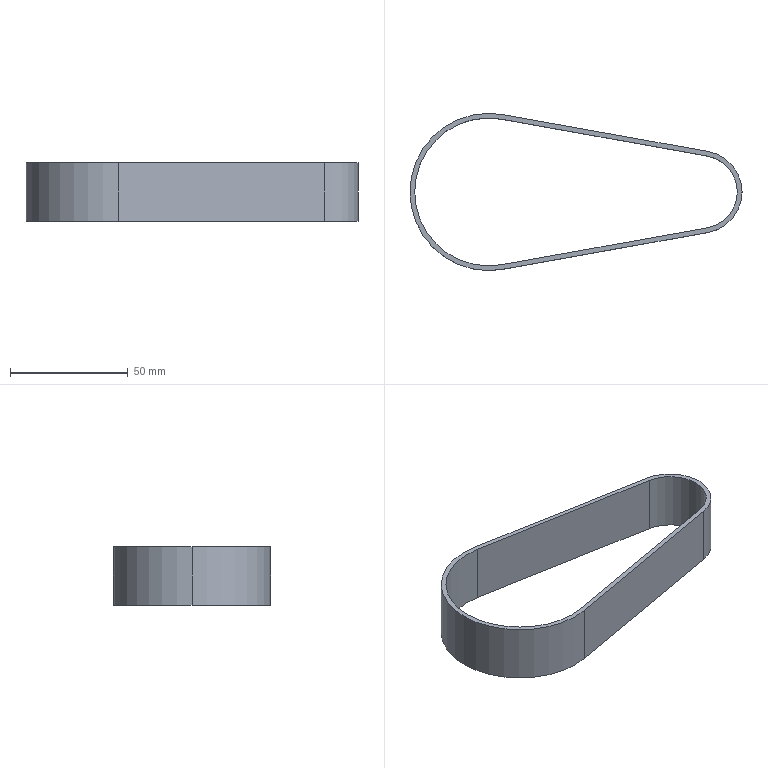Part | SolidWorks | features BaseBody 1 | 1 solid | 12 faces | box 140.79 x 66.7 x 25 mm | volume 16805 mm3 | cylinder 6 | plane 6 | commonest cylinder face diameters 62.7 x2 66.7 x2 30.88 x1 34.88 x1
STEP:
#1=CARTESIAN_POINT('',(-212.674,0.,25.));
#2=VERTEX_POINT('',#1);
#3=CARTESIAN_POINT('',(-175.782,30.856,25.));
#4=VERTEX_POINT('',#3);
#5=CARTESIAN_POINT('',(-181.324,0.,25.));
#6=DIRECTION('',(0.,0.,-1.));
#7=DIRECTION('',(-1.,0.,0.));
#8=AXIS2_PLACEMENT_3D('',#5,#6,#7);
#9=CIRCLE('',#8,31.35);
#10=EDGE_CURVE('',#2,#4,#9,.T.);
#11=ORIENTED_EDGE('',*,*,#10,.F.);
#12=CARTESIAN_POINT('',(-212.674,0.,0.));
#13=VERTEX_POINT('',#12);
#14=CARTESIAN_POINT('',(-212.674,0.,25.));
#15=DIRECTION('',(0.,0.,-1.));
#16=VECTOR('',#15,1000.);
#17=LINE('',#14,#16);
#18=EDGE_CURVE('',#2,#13,#17,.T.);
#19=ORIENTED_EDGE('',*,*,#18,.T.);
#20=CARTESIAN_POINT('',(-175.782,30.856,0.));
#21=VERTEX_POINT('',#20);
#22=CARTESIAN_POINT('',(-181.324,0.,0.));
#23=DIRECTION('',(0.,0.,1.));
#24=DIRECTION('',(-1.,0.,0.));
#25=AXIS2_PLACEMENT_3D('',#22,#23,#24);
#26=CIRCLE('',#25,31.35);
#27=EDGE_CURVE('',#21,#13,#26,.T.);
#28=ORIENTED_EDGE('',*,*,#27,.F.);
#29=CARTESIAN_POINT('',(-175.782,30.856,25.));
#30=DIRECTION('',(0.,0.,-1.));
#31=VECTOR('',#30,1000.);
#32=LINE('',#29,#31);
#33=EDGE_CURVE('',#4,#21,#32,.T.);
#34=ORIENTED_EDGE('',*,*,#33,.F.);
#35=EDGE_LOOP('',(#11,#19,#28,#34));
#36=FACE_OUTER_BOUND('',#35,.T.);
#37=CARTESIAN_POINT('',(-181.324,0.,25.));
#38=DIRECTION('',(0.,0.,-1.));
#39=DIRECTION('',(-1.,0.,0.));
#40=AXIS2_PLACEMENT_3D('',#37,#38,#39);
#41=CYLINDRICAL_SURFACE('',#40,31.35);
#42=ADVANCED_FACE('',(#36),#41,.F.);
#43=CARTESIAN_POINT('',(-214.674,0.,25.));
#44=VERTEX_POINT('',#43);
#45=CARTESIAN_POINT('',(-175.428,-32.825,25.));
#46=VERTEX_POINT('',#45);
#47=CARTESIAN_POINT('',(-181.324,0.,25.));
#48=DIRECTION('',(0.,0.,1.));
#49=DIRECTION('',(-1.,0.,0.));
#50=AXIS2_PLACEMENT_3D('',#47,#48,#49);
#51=CIRCLE('',#50,33.35);
#52=EDGE_CURVE('',#44,#46,#51,.T.);
#53=ORIENTED_EDGE('',*,*,#52,.F.);
#54=CARTESIAN_POINT('',(-214.674,0.,0.));
#55=VERTEX_POINT('',#54);
#56=CARTESIAN_POINT('',(-214.674,0.,25.));
#57=DIRECTION('',(0.,0.,-1.));
#58=VECTOR('',#57,1000.);
#59=LINE('',#56,#58);
#60=EDGE_CURVE('',#44,#55,#59,.T.);
#61=ORIENTED_EDGE('',*,*,#60,.T.);
#62=CARTESIAN_POINT('',(-175.428,-32.825,0.));
#63=VERTEX_POINT('',#62);
#64=CARTESIAN_POINT('',(-181.324,0.,0.));
#65=DIRECTION('',(0.,0.,1.));
#66=DIRECTION('',(-1.,0.,0.));
#67=AXIS2_PLACEMENT_3D('',#64,#65,#66);
#68=CIRCLE('',#67,33.35);
#69=EDGE_CURVE('',#55,#63,#68,.T.);
#70=ORIENTED_EDGE('',*,*,#69,.T.);
#71=CARTESIAN_POINT('',(-175.428,-32.825,25.));
#72=DIRECTION('',(0.,0.,1.));
#73=VECTOR('',#72,1000.);
#74=LINE('',#71,#73);
#75=EDGE_CURVE('',#63,#46,#74,.T.);
#76=ORIENTED_EDGE('',*,*,#75,.T.);
#77=EDGE_LOOP('',(#53,#61,#70,#76));
#78=FACE_OUTER_BOUND('',#77,.T.);
#79=CARTESIAN_POINT('',(-181.324,0.,25.));
#80=DIRECTION('',(0.,0.,-1.));
#81=DIRECTION('',(-1.,0.,0.));
#82=AXIS2_PLACEMENT_3D('',#79,#80,#81);
#83=CYLINDRICAL_SURFACE('',#82,33.35);
#84=ADVANCED_FACE('',(#78),#83,.T.);
#85=CARTESIAN_POINT('',(-175.782,-30.856,25.));
#86=VERTEX_POINT('',#85);
#87=CARTESIAN_POINT('',(-88.594,-15.197,25.));
#88=VERTEX_POINT('',#87);
#89=CARTESIAN_POINT('',(-175.782,-30.856,25.));
#90=DIRECTION('',(0.9843,0.1768,0.));
#91=VECTOR('',#90,1000.);
#92=LINE('',#89,#91);
#93=EDGE_CURVE('',#86,#88,#92,.T.);
#94=ORIENTED_EDGE('',*,*,#93,.T.);
#95=CARTESIAN_POINT('',(-88.594,-15.197,0.));
#96=VERTEX_POINT('',#95);
#97=CARTESIAN_POINT('',(-88.594,-15.197,25.));
#98=DIRECTION('',(0.,0.,-1.));
#99=VECTOR('',#98,1000.);
#100=LINE('',#97,#99);
#101=EDGE_CURVE('',#88,#96,#100,.T.);
#102=ORIENTED_EDGE('',*,*,#101,.T.);
#103=CARTESIAN_POINT('',(-175.782,-30.856,0.));
#104=VERTEX_POINT('',#103);
#105=CARTESIAN_POINT('',(-175.782,-30.856,0.));
#106=DIRECTION('',(-0.9843,-0.1768,0.));
#107=VECTOR('',#106,1000.);
#108=LINE('',#105,#107);
#109=EDGE_CURVE('',#96,#104,#108,.T.);
#110=ORIENTED_EDGE('',*,*,#109,.T.);
#111=CARTESIAN_POINT('',(-175.782,-30.856,25.));
#112=DIRECTION('',(0.,0.,1.));
#113=VECTOR('',#112,1000.);
#114=LINE('',#111,#113);
#115=EDGE_CURVE('',#104,#86,#114,.T.);
#116=ORIENTED_EDGE('',*,*,#115,.T.);
#117=EDGE_LOOP('',(#94,#102,#110,#116));
#118=FACE_OUTER_BOUND('',#117,.T.);
#119=CARTESIAN_POINT('',(-175.782,-30.856,25.));
#120=DIRECTION('',(-0.1768,0.9843,0.));
#121=DIRECTION('',(-0.9843,-0.1768,0.));
#122=AXIS2_PLACEMENT_3D('',#119,#120,#121);
#123=PLANE('',#122);
#124=ADVANCED_FACE('',(#118),#123,.T.);
#125=ORIENTED_EDGE('',*,*,#101,.F.);
#126=CARTESIAN_POINT('',(-88.594,15.197,25.));
#127=VERTEX_POINT('',#126);
#128=CARTESIAN_POINT('',(-91.324,0.,25.));
#129=DIRECTION('',(0.,0.,-1.));
#130=DIRECTION('',(-1.,0.,0.));
#131=AXIS2_PLACEMENT_3D('',#128,#129,#130);
#132=CIRCLE('',#131,15.44);
#133=EDGE_CURVE('',#127,#88,#132,.T.);
#134=ORIENTED_EDGE('',*,*,#133,.F.);
#135=CARTESIAN_POINT('',(-88.594,15.197,0.));
#136=VERTEX_POINT('',#135);
#137=CARTESIAN_POINT('',(-88.594,15.197,25.));
#138=DIRECTION('',(0.,0.,1.));
#139=VECTOR('',#138,1000.);
#140=LINE('',#137,#139);
#141=EDGE_CURVE('',#136,#127,#140,.T.);
#142=ORIENTED_EDGE('',*,*,#141,.F.);
#143=CARTESIAN_POINT('',(-91.324,0.,0.));
#144=DIRECTION('',(0.,0.,1.));
#145=DIRECTION('',(-1.,0.,0.));
#146=AXIS2_PLACEMENT_3D('',#143,#144,#145);
#147=CIRCLE('',#146,15.44);
#148=EDGE_CURVE('',#96,#136,#147,.T.);
#149=ORIENTED_EDGE('',*,*,#148,.F.);
#150=EDGE_LOOP('',(#125,#134,#142,#149));
#151=FACE_OUTER_BOUND('',#150,.T.);
#152=CARTESIAN_POINT('',(-91.324,0.,25.));
#153=DIRECTION('',(0.,0.,-1.));
#154=DIRECTION('',(-1.,0.,0.));
#155=AXIS2_PLACEMENT_3D('',#152,#153,#154);
#156=CYLINDRICAL_SURFACE('',#155,15.44);
#157=ADVANCED_FACE('',(#151),#156,.F.);
#158=CARTESIAN_POINT('',(-175.782,30.856,25.));
#159=DIRECTION('',(0.9843,-0.1768,0.));
#160=VECTOR('',#159,1000.);
#161=LINE('',#158,#160);
#162=EDGE_CURVE('',#4,#127,#161,.T.);
#163=ORIENTED_EDGE('',*,*,#162,.T.);
#164=ORIENTED_EDGE('',*,*,#133,.T.);
#165=ORIENTED_EDGE('',*,*,#93,.F.);
#166=CARTESIAN_POINT('',(-181.324,0.,25.));
#167=DIRECTION('',(0.,0.,-1.));
#168=DIRECTION('',(-1.,0.,0.));
#169=AXIS2_PLACEMENT_3D('',#166,#167,#168);
#170=CIRCLE('',#169,31.35);
#171=EDGE_CURVE('',#86,#2,#170,.T.);
#172=ORIENTED_EDGE('',*,*,#171,.T.);
#173=ORIENTED_EDGE('',*,*,#10,.T.);
#174=EDGE_LOOP('',(#163,#164,#165,#172,#173));
#175=FACE_BOUND('',#174,.T.);
#176=CARTESIAN_POINT('',(-88.241,-17.165,25.));
#177=VERTEX_POINT('',#176);
#178=CARTESIAN_POINT('',(-88.241,17.165,25.));
#179=VERTEX_POINT('',#178);
#180=CARTESIAN_POINT('',(-91.324,0.,25.));
#181=DIRECTION('',(0.,0.,1.));
#182=DIRECTION('',(-1.,0.,0.));
#183=AXIS2_PLACEMENT_3D('',#180,#181,#182);
#184=CIRCLE('',#183,17.44);
#185=EDGE_CURVE('',#177,#179,#184,.T.);
#186=ORIENTED_EDGE('',*,*,#185,.T.);
#187=CARTESIAN_POINT('',(-175.428,32.825,25.));
#188=VERTEX_POINT('',#187);
#189=CARTESIAN_POINT('',(-88.241,17.165,25.));
#190=DIRECTION('',(-0.9843,0.1768,0.));
#191=VECTOR('',#190,1000.);
#192=LINE('',#189,#191);
#193=EDGE_CURVE('',#179,#188,#192,.T.);
#194=ORIENTED_EDGE('',*,*,#193,.T.);
#195=CARTESIAN_POINT('',(-181.324,0.,25.));
#196=DIRECTION('',(0.,0.,1.));
#197=DIRECTION('',(-1.,0.,0.));
#198=AXIS2_PLACEMENT_3D('',#195,#196,#197);
#199=CIRCLE('',#198,33.35);
#200=EDGE_CURVE('',#188,#44,#199,.T.);
#201=ORIENTED_EDGE('',*,*,#200,.T.);
#202=ORIENTED_EDGE('',*,*,#52,.T.);
#203=CARTESIAN_POINT('',(-175.428,-32.825,25.));
#204=DIRECTION('',(0.9843,0.1768,0.));
#205=VECTOR('',#204,1000.);
#206=LINE('',#203,#205);
#207=EDGE_CURVE('',#46,#177,#206,.T.);
#208=ORIENTED_EDGE('',*,*,#207,.T.);
#209=EDGE_LOOP('',(#186,#194,#201,#202,#208));
#210=FACE_OUTER_BOUND('',#209,.T.);
#211=CARTESIAN_POINT('',(-181.324,0.,25.));
#212=DIRECTION('',(0.,0.,1.));
#213=DIRECTION('',(1.,0.,0.));
#214=AXIS2_PLACEMENT_3D('',#211,#212,#213);
#215=PLANE('',#214);
#216=ADVANCED_FACE('',(#175,#210),#215,.T.);
#217=ORIENTED_EDGE('',*,*,#18,.F.);
#218=ORIENTED_EDGE('',*,*,#171,.F.);
#219=ORIENTED_EDGE('',*,*,#115,.F.);
#220=CARTESIAN_POINT('',(-181.324,0.,0.));
#221=DIRECTION('',(0.,0.,1.));
#222=DIRECTION('',(-1.,0.,0.));
#223=AXIS2_PLACEMENT_3D('',#220,#221,#222);
#224=CIRCLE('',#223,31.35);
#225=EDGE_CURVE('',#13,#104,#224,.T.);
#226=ORIENTED_EDGE('',*,*,#225,.F.);
#227=EDGE_LOOP('',(#217,#218,#219,#226));
#228=FACE_OUTER_BOUND('',#227,.T.);
#229=CARTESIAN_POINT('',(-181.324,0.,25.));
#230=DIRECTION('',(0.,0.,-1.));
#231=DIRECTION('',(-1.,0.,0.));
#232=AXIS2_PLACEMENT_3D('',#229,#230,#231);
#233=CYLINDRICAL_SURFACE('',#232,31.35);
#234=ADVANCED_FACE('',(#228),#233,.F.);
#235=ORIENTED_EDGE('',*,*,#27,.T.);
#236=ORIENTED_EDGE('',*,*,#225,.T.);
#237=ORIENTED_EDGE('',*,*,#109,.F.);
#238=ORIENTED_EDGE('',*,*,#148,.T.);
#239=CARTESIAN_POINT('',(-175.782,30.856,0.));
#240=DIRECTION('',(0.9843,-0.1768,0.));
#241=VECTOR('',#240,1000.);
#242=LINE('',#239,#241);
#243=EDGE_CURVE('',#21,#136,#242,.T.);
#244=ORIENTED_EDGE('',*,*,#243,.F.);
#245=EDGE_LOOP('',(#235,#236,#237,#238,#244));
#246=FACE_BOUND('',#245,.T.);
#247=CARTESIAN_POINT('',(-88.241,17.165,0.));
#248=VERTEX_POINT('',#247);
#249=CARTESIAN_POINT('',(-175.428,32.825,0.));
#250=VERTEX_POINT('',#249);
#251=CARTESIAN_POINT('',(-88.241,17.165,0.));
#252=DIRECTION('',(-0.9843,0.1768,0.));
#253=VECTOR('',#252,1000.);
#254=LINE('',#251,#253);
#255=EDGE_CURVE('',#248,#250,#254,.T.);
#256=ORIENTED_EDGE('',*,*,#255,.F.);
#257=CARTESIAN_POINT('',(-88.241,-17.165,0.));
#258=VERTEX_POINT('',#257);
#259=CARTESIAN_POINT('',(-91.324,0.,0.));
#260=DIRECTION('',(0.,0.,1.));
#261=DIRECTION('',(-1.,0.,0.));
#262=AXIS2_PLACEMENT_3D('',#259,#260,#261);
#263=CIRCLE('',#262,17.44);
#264=EDGE_CURVE('',#258,#248,#263,.T.);
#265=ORIENTED_EDGE('',*,*,#264,.F.);
#266=CARTESIAN_POINT('',(-175.428,-32.825,0.));
#267=DIRECTION('',(0.9843,0.1768,0.));
#268=VECTOR('',#267,1000.);
#269=LINE('',#266,#268);
#270=EDGE_CURVE('',#63,#258,#269,.T.);
#271=ORIENTED_EDGE('',*,*,#270,.F.);
#272=ORIENTED_EDGE('',*,*,#69,.F.);
#273=CARTESIAN_POINT('',(-181.324,0.,0.));
#274=DIRECTION('',(0.,0.,1.));
#275=DIRECTION('',(-1.,0.,0.));
#276=AXIS2_PLACEMENT_3D('',#273,#274,#275);
#277=CIRCLE('',#276,33.35);
#278=EDGE_CURVE('',#250,#55,#277,.T.);
#279=ORIENTED_EDGE('',*,*,#278,.F.);
#280=EDGE_LOOP('',(#256,#265,#271,#272,#279));
#281=FACE_OUTER_BOUND('',#280,.T.);
#282=CARTESIAN_POINT('',(-181.324,0.,0.));
#283=DIRECTION('',(0.,0.,1.));
#284=DIRECTION('',(1.,0.,0.));
#285=AXIS2_PLACEMENT_3D('',#282,#283,#284);
#286=PLANE('',#285);
#287=ADVANCED_FACE('',(#246,#281),#286,.F.);
#288=ORIENTED_EDGE('',*,*,#162,.F.);
#289=ORIENTED_EDGE('',*,*,#33,.T.);
#290=ORIENTED_EDGE('',*,*,#243,.T.);
#291=ORIENTED_EDGE('',*,*,#141,.T.);
#292=EDGE_LOOP('',(#288,#289,#290,#291));
#293=FACE_OUTER_BOUND('',#292,.T.);
#294=CARTESIAN_POINT('',(-175.782,30.856,25.));
#295=DIRECTION('',(-0.1768,-0.9843,0.));
#296=DIRECTION('',(0.9843,-0.1768,0.));
#297=AXIS2_PLACEMENT_3D('',#294,#295,#296);
#298=PLANE('',#297);
#299=ADVANCED_FACE('',(#293),#298,.T.);
#300=CARTESIAN_POINT('',(-175.428,32.825,25.));
#301=DIRECTION('',(0.,0.,-1.));
#302=VECTOR('',#301,1000.);
#303=LINE('',#300,#302);
#304=EDGE_CURVE('',#188,#250,#303,.T.);
#305=ORIENTED_EDGE('',*,*,#304,.F.);
#306=ORIENTED_EDGE('',*,*,#193,.F.);
#307=CARTESIAN_POINT('',(-88.241,17.165,25.));
#308=DIRECTION('',(0.,0.,1.));
#309=VECTOR('',#308,1000.);
#310=LINE('',#307,#309);
#311=EDGE_CURVE('',#248,#179,#310,.T.);
#312=ORIENTED_EDGE('',*,*,#311,.F.);
#313=ORIENTED_EDGE('',*,*,#255,.T.);
#314=EDGE_LOOP('',(#305,#306,#312,#313));
#315=FACE_OUTER_BOUND('',#314,.T.);
#316=CARTESIAN_POINT('',(-175.428,32.825,25.));
#317=DIRECTION('',(-0.1768,-0.9843,0.));
#318=DIRECTION('',(0.9843,-0.1768,0.));
#319=AXIS2_PLACEMENT_3D('',#316,#317,#318);
#320=PLANE('',#319);
#321=ADVANCED_FACE('',(#315),#320,.F.);
#322=ORIENTED_EDGE('',*,*,#185,.F.);
#323=CARTESIAN_POINT('',(-88.241,-17.165,25.));
#324=DIRECTION('',(0.,0.,-1.));
#325=VECTOR('',#324,1000.);
#326=LINE('',#323,#325);
#327=EDGE_CURVE('',#177,#258,#326,.T.);
#328=ORIENTED_EDGE('',*,*,#327,.T.);
#329=ORIENTED_EDGE('',*,*,#264,.T.);
#330=ORIENTED_EDGE('',*,*,#311,.T.);
#331=EDGE_LOOP('',(#322,#328,#329,#330));
#332=FACE_OUTER_BOUND('',#331,.T.);
#333=CARTESIAN_POINT('',(-91.324,0.,25.));
#334=DIRECTION('',(0.,0.,-1.));
#335=DIRECTION('',(-1.,0.,0.));
#336=AXIS2_PLACEMENT_3D('',#333,#334,#335);
#337=CYLINDRICAL_SURFACE('',#336,17.44);
#338=ADVANCED_FACE('',(#332),#337,.T.);
#339=ORIENTED_EDGE('',*,*,#327,.F.);
#340=ORIENTED_EDGE('',*,*,#207,.F.);
#341=ORIENTED_EDGE('',*,*,#75,.F.);
#342=ORIENTED_EDGE('',*,*,#270,.T.);
#343=EDGE_LOOP('',(#339,#340,#341,#342));
#344=FACE_OUTER_BOUND('',#343,.T.);
#345=CARTESIAN_POINT('',(-175.428,-32.825,25.));
#346=DIRECTION('',(-0.1768,0.9843,0.));
#347=DIRECTION('',(-0.9843,-0.1768,0.));
#348=AXIS2_PLACEMENT_3D('',#345,#346,#347);
#349=PLANE('',#348);
#350=ADVANCED_FACE('',(#344),#349,.F.);
#351=ORIENTED_EDGE('',*,*,#60,.F.);
#352=ORIENTED_EDGE('',*,*,#200,.F.);
#353=ORIENTED_EDGE('',*,*,#304,.T.);
#354=ORIENTED_EDGE('',*,*,#278,.T.);
#355=EDGE_LOOP('',(#351,#352,#353,#354));
#356=FACE_OUTER_BOUND('',#355,.T.);
#357=CARTESIAN_POINT('',(-181.324,0.,25.));
#358=DIRECTION('',(0.,0.,-1.));
#359=DIRECTION('',(-1.,0.,0.));
#360=AXIS2_PLACEMENT_3D('',#357,#358,#359);
#361=CYLINDRICAL_SURFACE('',#360,33.35);
#362=ADVANCED_FACE('',(#356),#361,.T.);
#363=CLOSED_SHELL('',(#42,#84,#124,#157,#216,#234,#287,#299,#321,#338,#350,#362));
#364=MANIFOLD_SOLID_BREP('',#363);
#365=CARTESIAN_POINT('',(0.,0.,0.));
#366=DIRECTION('',(0.,0.,1.));
#367=DIRECTION('',(1.,0.,0.));
#368=AXIS2_PLACEMENT_3D('',#365,#366,#367);
#369=(LENGTH_UNIT()NAMED_UNIT(*)SI_UNIT(.MILLI.,.METRE.));
#370=UNCERTAINTY_MEASURE_WITH_UNIT(LENGTH_MEASURE(0.00001),#369,'','');
#371=(NAMED_UNIT(*)PLANE_ANGLE_UNIT()SI_UNIT($,.RADIAN.));
#372=(NAMED_UNIT(*)SI_UNIT($,.STERADIAN.)SOLID_ANGLE_UNIT());
#373=(GEOMETRIC_REPRESENTATION_CONTEXT(3)GLOBAL_UNCERTAINTY_ASSIGNED_CONTEXT((#370))GLOBAL_UNIT_ASSIGNED_CONTEXT((#369,#371,#372))REPRESENTATION_CONTEXT('',''));
#374=ADVANCED_BREP_SHAPE_REPRESENTATION('',(#364,#368),#373);